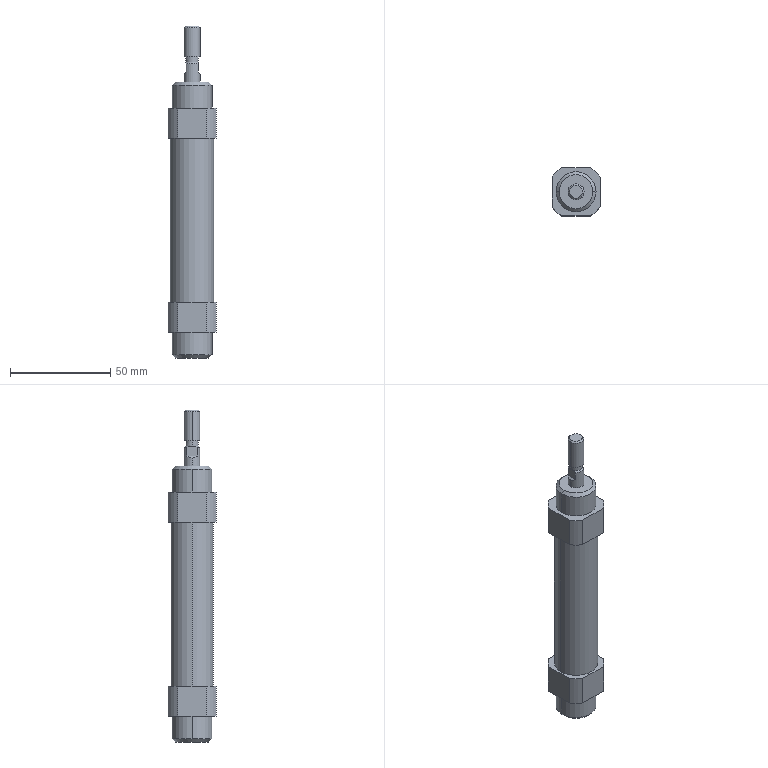Part | STEP file | CDM2B20-50-XC8 | 1 solid | 62 faces | box 24 x 24 x 166 mm | volume 54436 mm3 | cylinder 25 | plane 25 | cone 12 | commonest cylinder face diameters 28 x8 8 x5 8.57 x4 20 x4 6.47 x2 21.6 x2